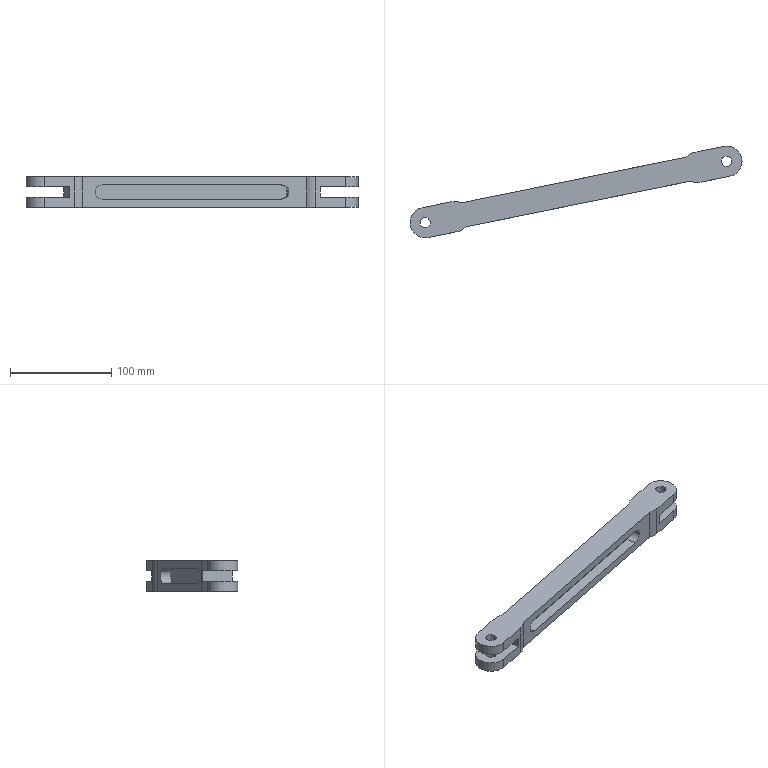Part | SolidWorks | features ICE 2, Extrusion 1, MirrorPattern 1 | 1 solid | 44 faces | box 327.343 x 90.496 x 30 mm | volume 173247 mm3 | cylinder 24 | plane 20 | commonest cylinder face diameters 30 x10 10 x8 14 x6
STEP:
#1=CARTESIAN_POINT('',(680.932,276.249,2993.336));
#2=VERTEX_POINT('',#1);
#3=CARTESIAN_POINT('',(674.073,274.853,2986.336));
#4=VERTEX_POINT('',#3);
#5=CARTESIAN_POINT('',(680.932,276.249,2986.336));
#6=DIRECTION('',(0.1994,-0.9799,0.));
#7=DIRECTION('',(0.9799,0.1994,0.));
#8=AXIS2_PLACEMENT_3D('',#5,#6,#7);
#9=CIRCLE('',#8,7.);
#10=EDGE_CURVE('',#2,#4,#9,.T.);
#11=ORIENTED_EDGE('',*,*,#10,.T.);
#12=CARTESIAN_POINT('',(672.079,284.652,2986.336));
#13=VERTEX_POINT('',#12);
#14=CARTESIAN_POINT('',(674.073,274.853,2986.336));
#15=DIRECTION('',(-0.1994,0.9799,0.));
#16=VECTOR('',#15,1000.);
#17=LINE('',#14,#16);
#18=EDGE_CURVE('',#4,#13,#17,.T.);
#19=ORIENTED_EDGE('',*,*,#18,.T.);
#20=CARTESIAN_POINT('',(678.939,286.048,2993.336));
#21=VERTEX_POINT('',#20);
#22=CARTESIAN_POINT('',(678.939,286.048,2986.336));
#23=DIRECTION('',(0.1994,-0.9799,0.));
#24=DIRECTION('',(0.9799,0.1994,0.));
#25=AXIS2_PLACEMENT_3D('',#22,#23,#24);
#26=CIRCLE('',#25,7.);
#27=EDGE_CURVE('',#21,#13,#26,.T.);
#28=ORIENTED_EDGE('',*,*,#27,.F.);
#29=CARTESIAN_POINT('',(680.932,276.249,2993.336));
#30=DIRECTION('',(-0.1994,0.9799,0.));
#31=VECTOR('',#30,1000.);
#32=LINE('',#29,#31);
#33=EDGE_CURVE('',#2,#21,#32,.T.);
#34=ORIENTED_EDGE('',*,*,#33,.F.);
#35=EDGE_LOOP('',(#11,#19,#28,#34));
#36=FACE_OUTER_BOUND('',#35,.T.);
#37=CARTESIAN_POINT('',(680.932,276.249,2986.336));
#38=DIRECTION('',(-0.1994,0.9799,0.));
#39=DIRECTION('',(-0.9799,-0.1994,0.));
#40=AXIS2_PLACEMENT_3D('',#37,#38,#39);
#41=CYLINDRICAL_SURFACE('',#40,7.);
#42=ADVANCED_FACE('',(#36),#41,.F.);
#43=CARTESIAN_POINT('',(865.742,309.767,2986.336));
#44=VERTEX_POINT('',#43);
#45=CARTESIAN_POINT('',(858.883,308.372,2993.336));
#46=VERTEX_POINT('',#45);
#47=CARTESIAN_POINT('',(858.883,308.372,2986.336));
#48=DIRECTION('',(0.1994,-0.9799,0.));
#49=DIRECTION('',(0.9799,0.1994,0.));
#50=AXIS2_PLACEMENT_3D('',#47,#48,#49);
#51=CIRCLE('',#50,7.);
#52=EDGE_CURVE('',#44,#46,#51,.T.);
#53=ORIENTED_EDGE('',*,*,#52,.F.);
#54=CARTESIAN_POINT('',(867.736,299.968,2986.336));
#55=VERTEX_POINT('',#54);
#56=CARTESIAN_POINT('',(865.742,309.767,2986.336));
#57=DIRECTION('',(0.1994,-0.9799,0.));
#58=VECTOR('',#57,1000.);
#59=LINE('',#56,#58);
#60=EDGE_CURVE('',#44,#55,#59,.T.);
#61=ORIENTED_EDGE('',*,*,#60,.T.);
#62=CARTESIAN_POINT('',(860.876,298.572,2993.336));
#63=VERTEX_POINT('',#62);
#64=CARTESIAN_POINT('',(860.876,298.572,2986.336));
#65=DIRECTION('',(0.1994,-0.9799,0.));
#66=DIRECTION('',(0.9799,0.1994,0.));
#67=AXIS2_PLACEMENT_3D('',#64,#65,#66);
#68=CIRCLE('',#67,7.);
#69=EDGE_CURVE('',#55,#63,#68,.T.);
#70=ORIENTED_EDGE('',*,*,#69,.T.);
#71=CARTESIAN_POINT('',(858.883,308.372,2993.336));
#72=DIRECTION('',(0.1994,-0.9799,0.));
#73=VECTOR('',#72,1000.);
#74=LINE('',#71,#73);
#75=EDGE_CURVE('',#46,#63,#74,.T.);
#76=ORIENTED_EDGE('',*,*,#75,.F.);
#77=EDGE_LOOP('',(#53,#61,#70,#76));
#78=FACE_OUTER_BOUND('',#77,.T.);
#79=CARTESIAN_POINT('',(858.883,308.372,2986.336));
#80=DIRECTION('',(0.1994,-0.9799,0.));
#81=DIRECTION('',(0.9799,0.1994,0.));
#82=AXIS2_PLACEMENT_3D('',#79,#80,#81);
#83=CYLINDRICAL_SURFACE('',#82,7.);
#84=ADVANCED_FACE('',(#78),#83,.F.);
#85=CARTESIAN_POINT('',(925.925,323.036,2991.336));
#86=VERTEX_POINT('',#85);
#87=CARTESIAN_POINT('',(915.925,323.036,2991.336));
#88=VERTEX_POINT('',#87);
#89=CARTESIAN_POINT('',(920.925,323.036,2991.336));
#90=DIRECTION('',(0.,0.,-1.));
#91=DIRECTION('',(1.,0.,0.));
#92=AXIS2_PLACEMENT_3D('',#89,#90,#91);
#93=CIRCLE('',#92,5.);
#94=EDGE_CURVE('',#86,#88,#93,.T.);
#95=ORIENTED_EDGE('',*,*,#94,.T.);
#96=CARTESIAN_POINT('',(915.925,323.036,3001.336));
#97=VERTEX_POINT('',#96);
#98=CARTESIAN_POINT('',(915.925,323.036,2631.714));
#99=DIRECTION('',(0.,0.,1.));
#100=VECTOR('',#99,1000.);
#101=LINE('',#98,#100);
#102=EDGE_CURVE('',#88,#97,#101,.T.);
#103=ORIENTED_EDGE('',*,*,#102,.T.);
#104=CARTESIAN_POINT('',(925.925,323.036,3001.336));
#105=VERTEX_POINT('',#104);
#106=CARTESIAN_POINT('',(920.925,323.036,3001.336));
#107=DIRECTION('',(0.,0.,1.));
#108=DIRECTION('',(1.,0.,0.));
#109=AXIS2_PLACEMENT_3D('',#106,#107,#108);
#110=CIRCLE('',#109,5.);
#111=EDGE_CURVE('',#97,#105,#110,.T.);
#112=ORIENTED_EDGE('',*,*,#111,.T.);
#113=CARTESIAN_POINT('',(925.925,323.036,2631.714));
#114=DIRECTION('',(0.,0.,1.));
#115=VECTOR('',#114,1000.);
#116=LINE('',#113,#115);
#117=EDGE_CURVE('',#86,#105,#116,.T.);
#118=ORIENTED_EDGE('',*,*,#117,.F.);
#119=EDGE_LOOP('',(#95,#103,#112,#118));
#120=FACE_OUTER_BOUND('',#119,.T.);
#121=CARTESIAN_POINT('',(920.925,323.036,2631.714));
#122=DIRECTION('',(0.,0.,1.));
#123=DIRECTION('',(1.,0.,0.));
#124=AXIS2_PLACEMENT_3D('',#121,#122,#123);
#125=CYLINDRICAL_SURFACE('',#124,5.);
#126=ADVANCED_FACE('',(#120),#125,.F.);
#127=CARTESIAN_POINT('',(628.582,262.54,2991.336));
#128=VERTEX_POINT('',#127);
#129=CARTESIAN_POINT('',(618.582,262.54,2991.336));
#130=VERTEX_POINT('',#129);
#131=CARTESIAN_POINT('',(623.582,262.54,2991.336));
#132=DIRECTION('',(0.,0.,-1.));
#133=DIRECTION('',(1.,0.,0.));
#134=AXIS2_PLACEMENT_3D('',#131,#132,#133);
#135=CIRCLE('',#134,5.);
#136=EDGE_CURVE('',#128,#130,#135,.T.);
#137=ORIENTED_EDGE('',*,*,#136,.T.);
#138=CARTESIAN_POINT('',(618.582,262.54,3001.336));
#139=VERTEX_POINT('',#138);
#140=CARTESIAN_POINT('',(618.582,262.54,2631.714));
#141=DIRECTION('',(0.,0.,1.));
#142=VECTOR('',#141,1000.);
#143=LINE('',#140,#142);
#144=EDGE_CURVE('',#130,#139,#143,.T.);
#145=ORIENTED_EDGE('',*,*,#144,.T.);
#146=CARTESIAN_POINT('',(628.582,262.54,3001.336));
#147=VERTEX_POINT('',#146);
#148=CARTESIAN_POINT('',(623.582,262.54,3001.336));
#149=DIRECTION('',(0.,0.,1.));
#150=DIRECTION('',(1.,0.,0.));
#151=AXIS2_PLACEMENT_3D('',#148,#149,#150);
#152=CIRCLE('',#151,5.);
#153=EDGE_CURVE('',#139,#147,#152,.T.);
#154=ORIENTED_EDGE('',*,*,#153,.T.);
#155=CARTESIAN_POINT('',(628.582,262.54,2631.714));
#156=DIRECTION('',(0.,0.,1.));
#157=VECTOR('',#156,1000.);
#158=LINE('',#155,#157);
#159=EDGE_CURVE('',#128,#147,#158,.T.);
#160=ORIENTED_EDGE('',*,*,#159,.F.);
#161=EDGE_LOOP('',(#137,#145,#154,#160));
#162=FACE_OUTER_BOUND('',#161,.T.);
#163=CARTESIAN_POINT('',(623.582,262.54,2631.714));
#164=DIRECTION('',(0.,0.,1.));
#165=DIRECTION('',(1.,0.,0.));
#166=AXIS2_PLACEMENT_3D('',#163,#164,#165);
#167=CYLINDRICAL_SURFACE('',#166,5.);
#168=ADVANCED_FACE('',(#162),#167,.F.);
#169=CARTESIAN_POINT('',(935.925,323.036,2991.336));
#170=VERTEX_POINT('',#169);
#171=CARTESIAN_POINT('',(923.916,308.337,2991.336));
#172=VERTEX_POINT('',#171);
#173=CARTESIAN_POINT('',(920.925,323.036,2991.336));
#174=DIRECTION('',(0.,0.,-1.));
#175=DIRECTION('',(1.,0.,0.));
#176=AXIS2_PLACEMENT_3D('',#173,#174,#175);
#177=CIRCLE('',#176,15.);
#178=EDGE_CURVE('',#170,#172,#177,.T.);
#179=ORIENTED_EDGE('',*,*,#178,.F.);
#180=CARTESIAN_POINT('',(935.925,323.036,3001.336));
#181=VERTEX_POINT('',#180);
#182=CARTESIAN_POINT('',(935.925,323.036,2631.714));
#183=DIRECTION('',(0.,0.,1.));
#184=VECTOR('',#183,1000.);
#185=LINE('',#182,#184);
#186=EDGE_CURVE('',#170,#181,#185,.T.);
#187=ORIENTED_EDGE('',*,*,#186,.T.);
#188=CARTESIAN_POINT('',(923.916,308.337,3001.336));
#189=VERTEX_POINT('',#188);
#190=CARTESIAN_POINT('',(920.925,323.036,3001.336));
#191=DIRECTION('',(0.,0.,1.));
#192=DIRECTION('',(1.,0.,0.));
#193=AXIS2_PLACEMENT_3D('',#190,#191,#192);
#194=CIRCLE('',#193,15.);
#195=EDGE_CURVE('',#189,#181,#194,.T.);
#196=ORIENTED_EDGE('',*,*,#195,.F.);
#197=CARTESIAN_POINT('',(923.916,308.337,2631.714));
#198=DIRECTION('',(0.,0.,1.));
#199=VECTOR('',#198,1000.);
#200=LINE('',#197,#199);
#201=EDGE_CURVE('',#172,#189,#200,.T.);
#202=ORIENTED_EDGE('',*,*,#201,.F.);
#203=EDGE_LOOP('',(#179,#187,#196,#202));
#204=FACE_OUTER_BOUND('',#203,.T.);
#205=CARTESIAN_POINT('',(920.925,323.036,2631.714));
#206=DIRECTION('',(0.,0.,1.));
#207=DIRECTION('',(1.,0.,0.));
#208=AXIS2_PLACEMENT_3D('',#205,#206,#207);
#209=CYLINDRICAL_SURFACE('',#208,15.);
#210=ADVANCED_FACE('',(#204),#209,.T.);
#211=CARTESIAN_POINT('',(925.925,323.036,2971.336));
#212=VERTEX_POINT('',#211);
#213=CARTESIAN_POINT('',(915.925,323.036,2971.336));
#214=VERTEX_POINT('',#213);
#215=CARTESIAN_POINT('',(920.925,323.036,2971.336));
#216=DIRECTION('',(0.,0.,-1.));
#217=DIRECTION('',(1.,0.,0.));
#218=AXIS2_PLACEMENT_3D('',#215,#216,#217);
#219=CIRCLE('',#218,5.);
#220=EDGE_CURVE('',#212,#214,#219,.T.);
#221=ORIENTED_EDGE('',*,*,#220,.T.);
#222=CARTESIAN_POINT('',(915.925,323.036,2981.336));
#223=VERTEX_POINT('',#222);
#224=CARTESIAN_POINT('',(915.925,323.036,2631.714));
#225=DIRECTION('',(0.,0.,1.));
#226=VECTOR('',#225,1000.);
#227=LINE('',#224,#226);
#228=EDGE_CURVE('',#214,#223,#227,.T.);
#229=ORIENTED_EDGE('',*,*,#228,.T.);
#230=CARTESIAN_POINT('',(925.925,323.036,2981.336));
#231=VERTEX_POINT('',#230);
#232=CARTESIAN_POINT('',(920.925,323.036,2981.336));
#233=DIRECTION('',(0.,0.,1.));
#234=DIRECTION('',(-1.,0.,0.));
#235=AXIS2_PLACEMENT_3D('',#232,#233,#234);
#236=CIRCLE('',#235,5.);
#237=EDGE_CURVE('',#223,#231,#236,.T.);
#238=ORIENTED_EDGE('',*,*,#237,.T.);
#239=CARTESIAN_POINT('',(925.925,323.036,2631.714));
#240=DIRECTION('',(0.,0.,1.));
#241=VECTOR('',#240,1000.);
#242=LINE('',#239,#241);
#243=EDGE_CURVE('',#212,#231,#242,.T.);
#244=ORIENTED_EDGE('',*,*,#243,.F.);
#245=EDGE_LOOP('',(#221,#229,#238,#244));
#246=FACE_OUTER_BOUND('',#245,.T.);
#247=CARTESIAN_POINT('',(920.925,323.036,2631.714));
#248=DIRECTION('',(0.,0.,1.));
#249=DIRECTION('',(1.,0.,0.));
#250=AXIS2_PLACEMENT_3D('',#247,#248,#249);
#251=CYLINDRICAL_SURFACE('',#250,5.);
#252=ADVANCED_FACE('',(#246),#251,.F.);
#253=CARTESIAN_POINT('',(628.582,262.54,2971.336));
#254=VERTEX_POINT('',#253);
#255=CARTESIAN_POINT('',(618.582,262.54,2971.336));
#256=VERTEX_POINT('',#255);
#257=CARTESIAN_POINT('',(623.582,262.54,2971.336));
#258=DIRECTION('',(0.,0.,-1.));
#259=DIRECTION('',(1.,0.,0.));
#260=AXIS2_PLACEMENT_3D('',#257,#258,#259);
#261=CIRCLE('',#260,5.);
#262=EDGE_CURVE('',#254,#256,#261,.T.);
#263=ORIENTED_EDGE('',*,*,#262,.T.);
#264=CARTESIAN_POINT('',(618.582,262.54,2981.336));
#265=VERTEX_POINT('',#264);
#266=CARTESIAN_POINT('',(618.582,262.54,2631.714));
#267=DIRECTION('',(0.,0.,1.));
#268=VECTOR('',#267,1000.);
#269=LINE('',#266,#268);
#270=EDGE_CURVE('',#256,#265,#269,.T.);
#271=ORIENTED_EDGE('',*,*,#270,.T.);
#272=CARTESIAN_POINT('',(628.582,262.54,2981.336));
#273=VERTEX_POINT('',#272);
#274=CARTESIAN_POINT('',(623.582,262.54,2981.336));
#275=DIRECTION('',(0.,0.,1.));
#276=DIRECTION('',(-1.,0.,0.));
#277=AXIS2_PLACEMENT_3D('',#274,#275,#276);
#278=CIRCLE('',#277,5.);
#279=EDGE_CURVE('',#265,#273,#278,.T.);
#280=ORIENTED_EDGE('',*,*,#279,.T.);
#281=CARTESIAN_POINT('',(628.582,262.54,2631.714));
#282=DIRECTION('',(0.,0.,1.));
#283=VECTOR('',#282,1000.);
#284=LINE('',#281,#283);
#285=EDGE_CURVE('',#254,#273,#284,.T.);
#286=ORIENTED_EDGE('',*,*,#285,.F.);
#287=EDGE_LOOP('',(#263,#271,#280,#286));
#288=FACE_OUTER_BOUND('',#287,.T.);
#289=CARTESIAN_POINT('',(623.582,262.54,2631.714));
#290=DIRECTION('',(0.,0.,1.));
#291=DIRECTION('',(1.,0.,0.));
#292=AXIS2_PLACEMENT_3D('',#289,#290,#291);
#293=CYLINDRICAL_SURFACE('',#292,5.);
#294=ADVANCED_FACE('',(#288),#293,.F.);
#295=CARTESIAN_POINT('',(935.925,323.036,2971.336));
#296=VERTEX_POINT('',#295);
#297=CARTESIAN_POINT('',(923.916,308.337,2971.336));
#298=VERTEX_POINT('',#297);
#299=CARTESIAN_POINT('',(920.925,323.036,2971.336));
#300=DIRECTION('',(0.,0.,-1.));
#301=DIRECTION('',(1.,0.,0.));
#302=AXIS2_PLACEMENT_3D('',#299,#300,#301);
#303=CIRCLE('',#302,15.);
#304=EDGE_CURVE('',#296,#298,#303,.T.);
#305=ORIENTED_EDGE('',*,*,#304,.F.);
#306=CARTESIAN_POINT('',(935.925,323.036,2981.336));
#307=VERTEX_POINT('',#306);
#308=CARTESIAN_POINT('',(935.925,323.036,2631.714));
#309=DIRECTION('',(0.,0.,1.));
#310=VECTOR('',#309,1000.);
#311=LINE('',#308,#310);
#312=EDGE_CURVE('',#296,#307,#311,.T.);
#313=ORIENTED_EDGE('',*,*,#312,.T.);
#314=CARTESIAN_POINT('',(923.916,308.337,2981.336));
#315=VERTEX_POINT('',#314);
#316=CARTESIAN_POINT('',(920.925,323.036,2981.336));
#317=DIRECTION('',(0.,0.,1.));
#318=DIRECTION('',(-1.,0.,0.));
#319=AXIS2_PLACEMENT_3D('',#316,#317,#318);
#320=CIRCLE('',#319,15.);
#321=EDGE_CURVE('',#315,#307,#320,.T.);
#322=ORIENTED_EDGE('',*,*,#321,.F.);
#323=CARTESIAN_POINT('',(923.916,308.337,2631.714));
#324=DIRECTION('',(0.,0.,1.));
#325=VECTOR('',#324,1000.);
#326=LINE('',#323,#325);
#327=EDGE_CURVE('',#298,#315,#326,.T.);
#328=ORIENTED_EDGE('',*,*,#327,.F.);
#329=EDGE_LOOP('',(#305,#313,#322,#328));
#330=FACE_OUTER_BOUND('',#329,.T.);
#331=CARTESIAN_POINT('',(920.925,323.036,2631.714));
#332=DIRECTION('',(0.,0.,1.));
#333=DIRECTION('',(1.,0.,0.));
#334=AXIS2_PLACEMENT_3D('',#331,#332,#333);
#335=CYLINDRICAL_SURFACE('',#334,15.);
#336=ADVANCED_FACE('',(#330),#335,.T.);
#337=CARTESIAN_POINT('',(659.407,282.074,2971.336));
#338=VERTEX_POINT('',#337);
#339=CARTESIAN_POINT('',(880.316,327.019,2971.336));
#340=VERTEX_POINT('',#339);
#341=CARTESIAN_POINT('',(880.316,327.019,2971.336));
#342=DIRECTION('',(0.9799,0.1994,0.));
#343=VECTOR('',#342,1000.);
#344=LINE('',#341,#343);
#345=EDGE_CURVE('',#338,#340,#344,.T.);
#346=ORIENTED_EDGE('',*,*,#345,.F.);
#347=CARTESIAN_POINT('',(659.407,282.074,3001.336));
#348=VERTEX_POINT('',#347);
#349=CARTESIAN_POINT('',(659.407,282.074,2631.714));
#350=DIRECTION('',(0.,0.,1.));
#351=VECTOR('',#350,1000.);
#352=LINE('',#349,#351);
#353=EDGE_CURVE('',#338,#348,#352,.T.);
#354=ORIENTED_EDGE('',*,*,#353,.T.);
#355=CARTESIAN_POINT('',(880.316,327.019,3001.336));
#356=VERTEX_POINT('',#355);
#357=CARTESIAN_POINT('',(880.316,327.019,3001.336));
#358=DIRECTION('',(-0.9799,-0.1994,0.));
#359=VECTOR('',#358,1000.);
#360=LINE('',#357,#359);
#361=EDGE_CURVE('',#356,#348,#360,.T.);
#362=ORIENTED_EDGE('',*,*,#361,.F.);
#363=CARTESIAN_POINT('',(880.316,327.019,2631.714));
#364=DIRECTION('',(0.,0.,1.));
#365=VECTOR('',#364,1000.);
#366=LINE('',#363,#365);
#367=EDGE_CURVE('',#340,#356,#366,.T.);
#368=ORIENTED_EDGE('',*,*,#367,.F.);
#369=EDGE_LOOP('',(#346,#354,#362,#368));
#370=FACE_OUTER_BOUND('',#369,.T.);
#371=CARTESIAN_POINT('',(856.091,322.091,2993.336));
#372=VERTEX_POINT('',#371);
#373=CARTESIAN_POINT('',(678.939,286.048,2993.336));
#374=DIRECTION('',(-0.9799,-0.1994,0.));
#375=VECTOR('',#374,1000.);
#376=LINE('',#373,#375);
#377=EDGE_CURVE('',#372,#21,#376,.T.);
#378=ORIENTED_EDGE('',*,*,#377,.T.);
#379=ORIENTED_EDGE('',*,*,#27,.T.);
#380=CARTESIAN_POINT('',(678.939,286.048,2979.336));
#381=VERTEX_POINT('',#380);
#382=CARTESIAN_POINT('',(678.939,286.048,2986.336));
#383=DIRECTION('',(0.1994,-0.9799,0.));
#384=DIRECTION('',(0.9799,0.1994,0.));
#385=AXIS2_PLACEMENT_3D('',#382,#383,#384);
#386=CIRCLE('',#385,7.);
#387=EDGE_CURVE('',#13,#381,#386,.T.);
#388=ORIENTED_EDGE('',*,*,#387,.T.);
#389=CARTESIAN_POINT('',(856.091,322.091,2979.336));
#390=VERTEX_POINT('',#389);
#391=CARTESIAN_POINT('',(678.939,286.048,2979.336));
#392=DIRECTION('',(0.9799,0.1994,0.));
#393=VECTOR('',#392,1000.);
#394=LINE('',#391,#393);
#395=EDGE_CURVE('',#381,#390,#394,.T.);
#396=ORIENTED_EDGE('',*,*,#395,.T.);
#397=CARTESIAN_POINT('',(856.091,322.091,2986.336));
#398=DIRECTION('',(0.1994,-0.9799,0.));
#399=DIRECTION('',(0.9799,0.1994,0.));
#400=AXIS2_PLACEMENT_3D('',#397,#398,#399);
#401=CIRCLE('',#400,7.);
#402=EDGE_CURVE('',#390,#372,#401,.T.);
#403=ORIENTED_EDGE('',*,*,#402,.T.);
#404=EDGE_LOOP('',(#378,#379,#388,#396,#403));
#405=FACE_BOUND('',#404,.T.);
#406=CARTESIAN_POINT('',(880.316,327.019,2631.714));
#407=DIRECTION('',(-0.1994,0.9799,0.));
#408=DIRECTION('',(-0.9799,-0.1994,0.));
#409=AXIS2_PLACEMENT_3D('',#406,#407,#408);
#410=PLANE('',#409);
#411=ADVANCED_FACE('',(#370,#405),#410,.T.);
#412=CARTESIAN_POINT('',(620.592,277.238,2981.336));
#413=VERTEX_POINT('',#412);
#414=CARTESIAN_POINT('',(626.573,247.841,2981.336));
#415=VERTEX_POINT('',#414);
#416=CARTESIAN_POINT('',(623.582,262.54,2981.336));
#417=DIRECTION('',(0.,0.,1.));
#418=DIRECTION('',(-1.,0.,0.));
#419=AXIS2_PLACEMENT_3D('',#416,#417,#418);
#420=CIRCLE('',#419,15.);
#421=EDGE_CURVE('',#413,#415,#420,.T.);
#422=ORIENTED_EDGE('',*,*,#421,.F.);
#423=CARTESIAN_POINT('',(620.592,277.238,2971.336));
#424=VERTEX_POINT('',#423);
#425=CARTESIAN_POINT('',(620.592,277.238,2631.714));
#426=DIRECTION('',(0.,0.,1.));
#427=VECTOR('',#426,1000.);
#428=LINE('',#425,#427);
#429=EDGE_CURVE('',#424,#413,#428,.T.);
#430=ORIENTED_EDGE('',*,*,#429,.F.);
#431=CARTESIAN_POINT('',(626.573,247.841,2971.336));
#432=VERTEX_POINT('',#431);
#433=CARTESIAN_POINT('',(623.582,262.54,2971.336));
#434=DIRECTION('',(0.,0.,-1.));
#435=DIRECTION('',(1.,0.,0.));
#436=AXIS2_PLACEMENT_3D('',#433,#434,#435);
#437=CIRCLE('',#436,15.);
#438=EDGE_CURVE('',#432,#424,#437,.T.);
#439=ORIENTED_EDGE('',*,*,#438,.F.);
#440=CARTESIAN_POINT('',(626.573,247.841,2631.714));
#441=DIRECTION('',(0.,0.,1.));
#442=VECTOR('',#441,1000.);
#443=LINE('',#440,#442);
#444=EDGE_CURVE('',#432,#415,#443,.T.);
#445=ORIENTED_EDGE('',*,*,#444,.T.);
#446=EDGE_LOOP('',(#422,#430,#439,#445));
#447=FACE_OUTER_BOUND('',#446,.T.);
#448=CARTESIAN_POINT('',(623.582,262.54,2631.714));
#449=DIRECTION('',(0.,0.,1.));
#450=DIRECTION('',(1.,0.,0.));
#451=AXIS2_PLACEMENT_3D('',#448,#449,#450);
#452=CYLINDRICAL_SURFACE('',#451,15.);
#453=ADVANCED_FACE('',(#447),#452,.T.);
#454=ORIENTED_EDGE('',*,*,#312,.F.);
#455=CARTESIAN_POINT('',(917.935,337.734,2971.336));
#456=VERTEX_POINT('',#455);
#457=CARTESIAN_POINT('',(920.925,323.036,2971.336));
#458=DIRECTION('',(0.,0.,-1.));
#459=DIRECTION('',(1.,0.,0.));
#460=AXIS2_PLACEMENT_3D('',#457,#458,#459);
#461=CIRCLE('',#460,15.);
#462=EDGE_CURVE('',#456,#296,#461,.T.);
#463=ORIENTED_EDGE('',*,*,#462,.F.);
#464=CARTESIAN_POINT('',(917.935,337.734,2981.336));
#465=VERTEX_POINT('',#464);
#466=CARTESIAN_POINT('',(917.935,337.734,2631.714));
#467=DIRECTION('',(0.,0.,1.));
#468=VECTOR('',#467,1000.);
#469=LINE('',#466,#468);
#470=EDGE_CURVE('',#456,#465,#469,.T.);
#471=ORIENTED_EDGE('',*,*,#470,.T.);
#472=CARTESIAN_POINT('',(920.925,323.036,2981.336));
#473=DIRECTION('',(0.,0.,1.));
#474=DIRECTION('',(-1.,0.,0.));
#475=AXIS2_PLACEMENT_3D('',#472,#473,#474);
#476=CIRCLE('',#475,15.);
#477=EDGE_CURVE('',#307,#465,#476,.T.);
#478=ORIENTED_EDGE('',*,*,#477,.F.);
#479=EDGE_LOOP('',(#454,#463,#471,#478));
#480=FACE_OUTER_BOUND('',#479,.T.);
#481=CARTESIAN_POINT('',(920.925,323.036,2631.714));
#482=DIRECTION('',(0.,0.,1.));
#483=DIRECTION('',(1.,0.,0.));
#484=AXIS2_PLACEMENT_3D('',#481,#482,#483);
#485=CYLINDRICAL_SURFACE('',#484,15.);
#486=ADVANCED_FACE('',(#480),#485,.T.);
#487=ORIENTED_EDGE('',*,*,#270,.F.);
#488=CARTESIAN_POINT('',(623.582,262.54,2971.336));
#489=DIRECTION('',(0.,0.,-1.));
#490=DIRECTION('',(1.,0.,0.));
#491=AXIS2_PLACEMENT_3D('',#488,#489,#490);
#492=CIRCLE('',#491,5.);
#493=EDGE_CURVE('',#256,#254,#492,.T.);
#494=ORIENTED_EDGE('',*,*,#493,.T.);
#495=ORIENTED_EDGE('',*,*,#285,.T.);
#496=CARTESIAN_POINT('',(623.582,262.54,2981.336));
#497=DIRECTION('',(0.,0.,1.));
#498=DIRECTION('',(-1.,0.,0.));
#499=AXIS2_PLACEMENT_3D('',#496,#497,#498);
#500=CIRCLE('',#499,5.);
#501=EDGE_CURVE('',#273,#265,#500,.T.);
#502=ORIENTED_EDGE('',*,*,#501,.T.);
#503=EDGE_LOOP('',(#487,#494,#495,#502));
#504=FACE_OUTER_BOUND('',#503,.T.);
#505=CARTESIAN_POINT('',(623.582,262.54,2631.714));
#506=DIRECTION('',(0.,0.,1.));
#507=DIRECTION('',(1.,0.,0.));
#508=AXIS2_PLACEMENT_3D('',#505,#506,#507);
#509=CYLINDRICAL_SURFACE('',#508,5.);
#510=ADVANCED_FACE('',(#504),#509,.F.);
#511=ORIENTED_EDGE('',*,*,#228,.F.);
#512=CARTESIAN_POINT('',(920.925,323.036,2971.336));
#513=DIRECTION('',(0.,0.,-1.));
#514=DIRECTION('',(1.,0.,0.));
#515=AXIS2_PLACEMENT_3D('',#512,#513,#514);
#516=CIRCLE('',#515,5.);
#517=EDGE_CURVE('',#214,#212,#516,.T.);
#518=ORIENTED_EDGE('',*,*,#517,.T.);
#519=ORIENTED_EDGE('',*,*,#243,.T.);
#520=CARTESIAN_POINT('',(920.925,323.036,2981.336));
#521=DIRECTION('',(0.,0.,1.));
#522=DIRECTION('',(-1.,0.,0.));
#523=AXIS2_PLACEMENT_3D('',#520,#521,#522);
#524=CIRCLE('',#523,5.);
#525=EDGE_CURVE('',#231,#223,#524,.T.);
#526=ORIENTED_EDGE('',*,*,#525,.T.);
#527=EDGE_LOOP('',(#511,#518,#519,#526));
#528=FACE_OUTER_BOUND('',#527,.T.);
#529=CARTESIAN_POINT('',(920.925,323.036,2631.714));
#530=DIRECTION('',(0.,0.,1.));
#531=DIRECTION('',(1.,0.,0.));
#532=AXIS2_PLACEMENT_3D('',#529,#530,#531);
#533=CYLINDRICAL_SURFACE('',#532,5.);
#534=ADVANCED_FACE('',(#528),#533,.F.);
#535=CARTESIAN_POINT('',(892.569,332.574,2981.336));
#536=VERTEX_POINT('',#535);
#537=CARTESIAN_POINT('',(917.935,337.734,2981.336));
#538=DIRECTION('',(-0.9799,-0.1994,0.));
#539=VECTOR('',#538,1000.);
#540=LINE('',#537,#539);
#541=EDGE_CURVE('',#465,#536,#540,.T.);
#542=ORIENTED_EDGE('',*,*,#541,.F.);
#543=ORIENTED_EDGE('',*,*,#470,.F.);
#544=CARTESIAN_POINT('',(888.537,331.753,2971.336));
#545=VERTEX_POINT('',#544);
#546=CARTESIAN_POINT('',(917.935,337.734,2971.336));
#547=DIRECTION('',(0.9799,0.1994,0.));
#548=VECTOR('',#547,1000.);
#549=LINE('',#546,#548);
#550=EDGE_CURVE('',#545,#456,#549,.T.);
#551=ORIENTED_EDGE('',*,*,#550,.F.);
#552=CARTESIAN_POINT('',(888.537,331.753,3001.336));
#553=VERTEX_POINT('',#552);
#554=CARTESIAN_POINT('',(888.537,331.753,2631.714));
#555=DIRECTION('',(0.,0.,1.));
#556=VECTOR('',#555,1000.);
#557=LINE('',#554,#556);
#558=EDGE_CURVE('',#545,#553,#557,.T.);
#559=ORIENTED_EDGE('',*,*,#558,.T.);
#560=CARTESIAN_POINT('',(917.935,337.734,3001.336));
#561=VERTEX_POINT('',#560);
#562=CARTESIAN_POINT('',(917.935,337.734,3001.336));
#563=DIRECTION('',(-0.9799,-0.1994,0.));
#564=VECTOR('',#563,1000.);
#565=LINE('',#562,#564);
#566=EDGE_CURVE('',#561,#553,#565,.T.);
#567=ORIENTED_EDGE('',*,*,#566,.F.);
#568=CARTESIAN_POINT('',(917.935,337.734,2991.336));
#569=VERTEX_POINT('',#568);
#570=CARTESIAN_POINT('',(917.935,337.734,2631.714));
#571=DIRECTION('',(0.,0.,1.));
#572=VECTOR('',#571,1000.);
#573=LINE('',#570,#572);
#574=EDGE_CURVE('',#569,#561,#573,.T.);
#575=ORIENTED_EDGE('',*,*,#574,.F.);
#576=CARTESIAN_POINT('',(892.569,332.574,2991.336));
#577=VERTEX_POINT('',#576);
#578=CARTESIAN_POINT('',(917.935,337.734,2991.336));
#579=DIRECTION('',(0.9799,0.1994,0.));
#580=VECTOR('',#579,1000.);
#581=LINE('',#578,#580);
#582=EDGE_CURVE('',#577,#569,#581,.T.);
#583=ORIENTED_EDGE('',*,*,#582,.F.);
#584=CARTESIAN_POINT('',(892.569,332.574,2631.714));
#585=DIRECTION('',(0.,0.,1.));
#586=VECTOR('',#585,1000.);
#587=LINE('',#584,#586);
#588=EDGE_CURVE('',#536,#577,#587,.T.);
#589=ORIENTED_EDGE('',*,*,#588,.F.);
#590=EDGE_LOOP('',(#542,#543,#551,#559,#567,#575,#583,#589));
#591=FACE_OUTER_BOUND('',#590,.T.);
#592=CARTESIAN_POINT('',(917.935,337.734,2631.714));
#593=DIRECTION('',(-0.1994,0.9799,0.));
#594=DIRECTION('',(-0.9799,-0.1994,0.));
#595=AXIS2_PLACEMENT_3D('',#592,#593,#594);
#596=PLANE('',#595);
#597=ADVANCED_FACE('',(#591),#596,.T.);
#598=CARTESIAN_POINT('',(891.528,317.054,2971.336));
#599=DIRECTION('',(0.,0.,-1.));
#600=DIRECTION('',(1.,0.,0.));
#601=AXIS2_PLACEMENT_3D('',#598,#599,#600);
#602=CIRCLE('',#601,15.);
#603=EDGE_CURVE('',#340,#545,#602,.T.);
#604=ORIENTED_EDGE('',*,*,#603,.F.);
#605=ORIENTED_EDGE('',*,*,#367,.T.);
#606=CARTESIAN_POINT('',(891.528,317.054,3001.336));
#607=DIRECTION('',(0.,0.,1.));
#608=DIRECTION('',(1.,0.,0.));
#609=AXIS2_PLACEMENT_3D('',#606,#607,#608);
#610=CIRCLE('',#609,15.);
#611=EDGE_CURVE('',#553,#356,#610,.T.);
#612=ORIENTED_EDGE('',*,*,#611,.F.);
#613=ORIENTED_EDGE('',*,*,#558,.F.);
#614=EDGE_LOOP('',(#604,#605,#612,#613));
#615=FACE_OUTER_BOUND('',#614,.T.);
#616=CARTESIAN_POINT('',(891.528,317.054,2631.714));
#617=DIRECTION('',(0.,0.,1.));
#618=DIRECTION('',(1.,0.,0.));
#619=AXIS2_PLACEMENT_3D('',#616,#617,#618);
#620=CYLINDRICAL_SURFACE('',#619,15.);
#621=ADVANCED_FACE('',(#615),#620,.T.);
#622=CARTESIAN_POINT('',(649.989,283.22,2971.336));
#623=VERTEX_POINT('',#622);
#624=CARTESIAN_POINT('',(652.98,268.521,2971.336));
#625=DIRECTION('',(0.,0.,-1.));
#626=DIRECTION('',(1.,0.,0.));
#627=AXIS2_PLACEMENT_3D('',#624,#625,#626);
#628=CIRCLE('',#627,15.);
#629=EDGE_CURVE('',#623,#338,#628,.T.);
#630=ORIENTED_EDGE('',*,*,#629,.F.);
#631=CARTESIAN_POINT('',(649.989,283.22,3001.336));
#632=VERTEX_POINT('',#631);
#633=CARTESIAN_POINT('',(649.989,283.22,2631.714));
#634=DIRECTION('',(0.,0.,1.));
#635=VECTOR('',#634,1000.);
#636=LINE('',#633,#635);
#637=EDGE_CURVE('',#623,#632,#636,.T.);
#638=ORIENTED_EDGE('',*,*,#637,.T.);
#639=CARTESIAN_POINT('',(652.98,268.521,3001.336));
#640=DIRECTION('',(0.,0.,1.));
#641=DIRECTION('',(1.,0.,0.));
#642=AXIS2_PLACEMENT_3D('',#639,#640,#641);
#643=CIRCLE('',#642,15.);
#644=EDGE_CURVE('',#348,#632,#643,.T.);
#645=ORIENTED_EDGE('',*,*,#644,.F.);
#646=ORIENTED_EDGE('',*,*,#353,.F.);
#647=EDGE_LOOP('',(#630,#638,#645,#646));
#648=FACE_OUTER_BOUND('',#647,.T.);
#649=CARTESIAN_POINT('',(652.98,268.521,2631.714));
#650=DIRECTION('',(0.,0.,1.));
#651=DIRECTION('',(1.,0.,0.));
#652=AXIS2_PLACEMENT_3D('',#649,#650,#651);
#653=CYLINDRICAL_SURFACE('',#652,15.);
#654=ADVANCED_FACE('',(#648),#653,.T.);
#655=CARTESIAN_POINT('',(645.957,282.399,2981.336));
#656=VERTEX_POINT('',#655);
#657=CARTESIAN_POINT('',(649.989,283.22,2981.336));
#658=DIRECTION('',(-0.9799,-0.1994,0.));
#659=VECTOR('',#658,1000.);
#660=LINE('',#657,#659);
#661=EDGE_CURVE('',#656,#413,#660,.T.);
#662=ORIENTED_EDGE('',*,*,#661,.F.);
#663=CARTESIAN_POINT('',(645.957,282.399,2991.336));
#664=VERTEX_POINT('',#663);
#665=CARTESIAN_POINT('',(645.957,282.399,2631.714));
#666=DIRECTION('',(0.,0.,-1.));
#667=VECTOR('',#666,1000.);
#668=LINE('',#665,#667);
#669=EDGE_CURVE('',#664,#656,#668,.T.);
#670=ORIENTED_EDGE('',*,*,#669,.F.);
#671=CARTESIAN_POINT('',(620.592,277.238,2991.336));
#672=VERTEX_POINT('',#671);
#673=CARTESIAN_POINT('',(649.989,283.22,2991.336));
#674=DIRECTION('',(0.9799,0.1994,0.));
#675=VECTOR('',#674,1000.);
#676=LINE('',#673,#675);
#677=EDGE_CURVE('',#672,#664,#676,.T.);
#678=ORIENTED_EDGE('',*,*,#677,.F.);
#679=CARTESIAN_POINT('',(620.592,277.238,3001.336));
#680=VERTEX_POINT('',#679);
#681=CARTESIAN_POINT('',(620.592,277.238,2631.714));
#682=DIRECTION('',(0.,0.,1.));
#683=VECTOR('',#682,1000.);
#684=LINE('',#681,#683);
#685=EDGE_CURVE('',#672,#680,#684,.T.);
#686=ORIENTED_EDGE('',*,*,#685,.T.);
#687=CARTESIAN_POINT('',(649.989,283.22,3001.336));
#688=DIRECTION('',(-0.9799,-0.1994,0.));
#689=VECTOR('',#688,1000.);
#690=LINE('',#687,#689);
#691=EDGE_CURVE('',#632,#680,#690,.T.);
#692=ORIENTED_EDGE('',*,*,#691,.F.);
#693=ORIENTED_EDGE('',*,*,#637,.F.);
#694=CARTESIAN_POINT('',(649.989,283.22,2971.336));
#695=DIRECTION('',(0.9799,0.1994,0.));
#696=VECTOR('',#695,1000.);
#697=LINE('',#694,#696);
#698=EDGE_CURVE('',#424,#623,#697,.T.);
#699=ORIENTED_EDGE('',*,*,#698,.F.);
#700=ORIENTED_EDGE('',*,*,#429,.T.);
#701=EDGE_LOOP('',(#662,#670,#678,#686,#692,#693,#699,#700));
#702=FACE_OUTER_BOUND('',#701,.T.);
#703=CARTESIAN_POINT('',(649.989,283.22,2631.714));
#704=DIRECTION('',(-0.1994,0.9799,0.));
#705=DIRECTION('',(-0.9799,-0.1994,0.));
#706=AXIS2_PLACEMENT_3D('',#703,#704,#705);
#707=PLANE('',#706);
#708=ADVANCED_FACE('',(#702),#707,.T.);
#709=CARTESIAN_POINT('',(626.573,247.841,2991.336));
#710=VERTEX_POINT('',#709);
#711=CARTESIAN_POINT('',(623.582,262.54,2991.336));
#712=DIRECTION('',(0.,0.,-1.));
#713=DIRECTION('',(1.,0.,0.));
#714=AXIS2_PLACEMENT_3D('',#711,#712,#713);
#715=CIRCLE('',#714,15.);
#716=EDGE_CURVE('',#710,#672,#715,.T.);
#717=ORIENTED_EDGE('',*,*,#716,.F.);
#718=CARTESIAN_POINT('',(626.573,247.841,3001.336));
#719=VERTEX_POINT('',#718);
#720=CARTESIAN_POINT('',(626.573,247.841,2631.714));
#721=DIRECTION('',(0.,0.,1.));
#722=VECTOR('',#721,1000.);
#723=LINE('',#720,#722);
#724=EDGE_CURVE('',#710,#719,#723,.T.);
#725=ORIENTED_EDGE('',*,*,#724,.T.);
#726=CARTESIAN_POINT('',(623.582,262.54,3001.336));
#727=DIRECTION('',(0.,0.,1.));
#728=DIRECTION('',(1.,0.,0.));
#729=AXIS2_PLACEMENT_3D('',#726,#727,#728);
#730=CIRCLE('',#729,15.);
#731=EDGE_CURVE('',#680,#719,#730,.T.);
#732=ORIENTED_EDGE('',*,*,#731,.F.);
#733=ORIENTED_EDGE('',*,*,#685,.F.);
#734=EDGE_LOOP('',(#717,#725,#732,#733));
#735=FACE_OUTER_BOUND('',#734,.T.);
#736=CARTESIAN_POINT('',(623.582,262.54,2631.714));
#737=DIRECTION('',(0.,0.,1.));
#738=DIRECTION('',(1.,0.,0.));
#739=AXIS2_PLACEMENT_3D('',#736,#737,#738);
#740=CYLINDRICAL_SURFACE('',#739,15.);
#741=ADVANCED_FACE('',(#735),#740,.T.);
#742=CARTESIAN_POINT('',(651.938,253.001,2981.336));
#743=VERTEX_POINT('',#742);
#744=CARTESIAN_POINT('',(651.938,253.001,2981.336));
#745=DIRECTION('',(0.9799,0.1994,0.));
#746=VECTOR('',#745,1000.);
#747=LINE('',#744,#746);
#748=EDGE_CURVE('',#415,#743,#747,.T.);
#749=ORIENTED_EDGE('',*,*,#748,.F.);
#750=ORIENTED_EDGE('',*,*,#444,.F.);
#751=CARTESIAN_POINT('',(655.97,253.822,2971.336));
#752=VERTEX_POINT('',#751);
#753=CARTESIAN_POINT('',(626.573,247.841,2971.336));
#754=DIRECTION('',(-0.9799,-0.1994,0.));
#755=VECTOR('',#754,1000.);
#756=LINE('',#753,#755);
#757=EDGE_CURVE('',#752,#432,#756,.T.);
#758=ORIENTED_EDGE('',*,*,#757,.F.);
#759=CARTESIAN_POINT('',(655.97,253.822,3001.336));
#760=VERTEX_POINT('',#759);
#761=CARTESIAN_POINT('',(655.97,253.822,2631.714));
#762=DIRECTION('',(0.,0.,1.));
#763=VECTOR('',#762,1000.);
#764=LINE('',#761,#763);
#765=EDGE_CURVE('',#752,#760,#764,.T.);
#766=ORIENTED_EDGE('',*,*,#765,.T.);
#767=CARTESIAN_POINT('',(626.573,247.841,3001.336));
#768=DIRECTION('',(0.9799,0.1994,0.));
#769=VECTOR('',#768,1000.);
#770=LINE('',#767,#769);
#771=EDGE_CURVE('',#719,#760,#770,.T.);
#772=ORIENTED_EDGE('',*,*,#771,.F.);
#773=ORIENTED_EDGE('',*,*,#724,.F.);
#774=CARTESIAN_POINT('',(651.938,253.001,2991.336));
#775=VERTEX_POINT('',#774);
#776=CARTESIAN_POINT('',(651.938,253.001,2991.336));
#777=DIRECTION('',(-0.9799,-0.1994,0.));
#778=VECTOR('',#777,1000.);
#779=LINE('',#776,#778);
#780=EDGE_CURVE('',#775,#710,#779,.T.);
#781=ORIENTED_EDGE('',*,*,#780,.F.);
#782=CARTESIAN_POINT('',(651.938,253.001,2991.336));
#783=DIRECTION('',(0.,0.,1.));
#784=VECTOR('',#783,1000.);
#785=LINE('',#782,#784);
#786=EDGE_CURVE('',#743,#775,#785,.T.);
#787=ORIENTED_EDGE('',*,*,#786,.F.);
#788=EDGE_LOOP('',(#749,#750,#758,#766,#772,#773,#781,#787));
#789=FACE_OUTER_BOUND('',#788,.T.);
#790=CARTESIAN_POINT('',(626.573,247.841,2631.714));
#791=DIRECTION('',(0.1994,-0.9799,0.));
#792=DIRECTION('',(0.9799,0.1994,0.));
#793=AXIS2_PLACEMENT_3D('',#790,#791,#792);
#794=PLANE('',#793);
#795=ADVANCED_FACE('',(#789),#794,.T.);
#796=CARTESIAN_POINT('',(664.192,258.556,2971.336));
#797=VERTEX_POINT('',#796);
#798=CARTESIAN_POINT('',(652.98,268.521,2971.336));
#799=DIRECTION('',(0.,0.,-1.));
#800=DIRECTION('',(1.,0.,0.));
#801=AXIS2_PLACEMENT_3D('',#798,#799,#800);
#802=CIRCLE('',#801,15.);
#803=EDGE_CURVE('',#797,#752,#802,.T.);
#804=ORIENTED_EDGE('',*,*,#803,.F.);
#805=CARTESIAN_POINT('',(664.192,258.556,3001.336));
#806=VERTEX_POINT('',#805);
#807=CARTESIAN_POINT('',(664.192,258.556,2631.714));
#808=DIRECTION('',(0.,0.,1.));
#809=VECTOR('',#808,1000.);
#810=LINE('',#807,#809);
#811=EDGE_CURVE('',#797,#806,#810,.T.);
#812=ORIENTED_EDGE('',*,*,#811,.T.);
#813=CARTESIAN_POINT('',(652.98,268.521,3001.336));
#814=DIRECTION('',(0.,0.,1.));
#815=DIRECTION('',(1.,0.,0.));
#816=AXIS2_PLACEMENT_3D('',#813,#814,#815);
#817=CIRCLE('',#816,15.);
#818=EDGE_CURVE('',#760,#806,#817,.T.);
#819=ORIENTED_EDGE('',*,*,#818,.F.);
#820=ORIENTED_EDGE('',*,*,#765,.F.);
#821=EDGE_LOOP('',(#804,#812,#819,#820));
#822=FACE_OUTER_BOUND('',#821,.T.);
#823=CARTESIAN_POINT('',(652.98,268.521,2631.714));
#824=DIRECTION('',(0.,0.,1.));
#825=DIRECTION('',(1.,0.,0.));
#826=AXIS2_PLACEMENT_3D('',#823,#824,#825);
#827=CYLINDRICAL_SURFACE('',#826,15.);
#828=ADVANCED_FACE('',(#822),#827,.T.);
#829=CARTESIAN_POINT('',(683.724,262.53,2993.336));
#830=VERTEX_POINT('',#829);
#831=CARTESIAN_POINT('',(683.724,262.53,2979.336));
#832=VERTEX_POINT('',#831);
#833=CARTESIAN_POINT('',(683.724,262.53,2986.336));
#834=DIRECTION('',(0.1994,-0.9799,0.));
#835=DIRECTION('',(0.9799,0.1994,0.));
#836=AXIS2_PLACEMENT_3D('',#833,#834,#835);
#837=CIRCLE('',#836,7.);
#838=EDGE_CURVE('',#830,#832,#837,.T.);
#839=ORIENTED_EDGE('',*,*,#838,.F.);
#840=CARTESIAN_POINT('',(683.724,262.53,2993.336));
#841=DIRECTION('',(-0.9799,-0.1994,0.));
#842=VECTOR('',#841,1000.);
#843=LINE('',#840,#842);
#844=EDGE_CURVE('',#63,#830,#843,.T.);
#845=ORIENTED_EDGE('',*,*,#844,.F.);
#846=ORIENTED_EDGE('',*,*,#69,.F.);
#847=CARTESIAN_POINT('',(860.876,298.572,2979.336));
#848=VERTEX_POINT('',#847);
#849=CARTESIAN_POINT('',(860.876,298.572,2986.336));
#850=DIRECTION('',(0.1994,-0.9799,0.));
#851=DIRECTION('',(0.9799,0.1994,0.));
#852=AXIS2_PLACEMENT_3D('',#849,#850,#851);
#853=CIRCLE('',#852,7.);
#854=EDGE_CURVE('',#848,#55,#853,.T.);
#855=ORIENTED_EDGE('',*,*,#854,.F.);
#856=CARTESIAN_POINT('',(683.724,262.53,2979.336));
#857=DIRECTION('',(0.9799,0.1994,0.));
#858=VECTOR('',#857,1000.);
#859=LINE('',#856,#858);
#860=EDGE_CURVE('',#832,#848,#859,.T.);
#861=ORIENTED_EDGE('',*,*,#860,.F.);
#862=EDGE_LOOP('',(#839,#845,#846,#855,#861));
#863=FACE_BOUND('',#862,.T.);
#864=CARTESIAN_POINT('',(885.101,303.501,2971.336));
#865=VERTEX_POINT('',#864);
#866=CARTESIAN_POINT('',(664.192,258.556,2971.336));
#867=DIRECTION('',(-0.9799,-0.1994,0.));
#868=VECTOR('',#867,1000.);
#869=LINE('',#866,#868);
#870=EDGE_CURVE('',#865,#797,#869,.T.);
#871=ORIENTED_EDGE('',*,*,#870,.F.);
#872=CARTESIAN_POINT('',(885.101,303.501,3001.336));
#873=VERTEX_POINT('',#872);
#874=CARTESIAN_POINT('',(885.101,303.501,2631.714));
#875=DIRECTION('',(0.,0.,1.));
#876=VECTOR('',#875,1000.);
#877=LINE('',#874,#876);
#878=EDGE_CURVE('',#865,#873,#877,.T.);
#879=ORIENTED_EDGE('',*,*,#878,.T.);
#880=CARTESIAN_POINT('',(664.192,258.556,3001.336));
#881=DIRECTION('',(0.9799,0.1994,0.));
#882=VECTOR('',#881,1000.);
#883=LINE('',#880,#882);
#884=EDGE_CURVE('',#806,#873,#883,.T.);
#885=ORIENTED_EDGE('',*,*,#884,.F.);
#886=ORIENTED_EDGE('',*,*,#811,.F.);
#887=EDGE_LOOP('',(#871,#879,#885,#886));
#888=FACE_OUTER_BOUND('',#887,.T.);
#889=CARTESIAN_POINT('',(664.192,258.556,2631.714));
#890=DIRECTION('',(0.1994,-0.9799,0.));
#891=DIRECTION('',(0.9799,0.1994,0.));
#892=AXIS2_PLACEMENT_3D('',#889,#890,#891);
#893=PLANE('',#892);
#894=ADVANCED_FACE('',(#863,#888),#893,.T.);
#895=CARTESIAN_POINT('',(894.518,302.356,2971.336));
#896=VERTEX_POINT('',#895);
#897=CARTESIAN_POINT('',(891.528,317.054,2971.336));
#898=DIRECTION('',(0.,0.,-1.));
#899=DIRECTION('',(1.,0.,0.));
#900=AXIS2_PLACEMENT_3D('',#897,#898,#899);
#901=CIRCLE('',#900,15.);
#902=EDGE_CURVE('',#896,#865,#901,.T.);
#903=ORIENTED_EDGE('',*,*,#902,.F.);
#904=CARTESIAN_POINT('',(894.518,302.356,3001.336));
#905=VERTEX_POINT('',#904);
#906=CARTESIAN_POINT('',(894.518,302.356,2631.714));
#907=DIRECTION('',(0.,0.,1.));
#908=VECTOR('',#907,1000.);
#909=LINE('',#906,#908);
#910=EDGE_CURVE('',#896,#905,#909,.T.);
#911=ORIENTED_EDGE('',*,*,#910,.T.);
#912=CARTESIAN_POINT('',(891.528,317.054,3001.336));
#913=DIRECTION('',(0.,0.,1.));
#914=DIRECTION('',(1.,0.,0.));
#915=AXIS2_PLACEMENT_3D('',#912,#913,#914);
#916=CIRCLE('',#915,15.);
#917=EDGE_CURVE('',#873,#905,#916,.T.);
#918=ORIENTED_EDGE('',*,*,#917,.F.);
#919=ORIENTED_EDGE('',*,*,#878,.F.);
#920=EDGE_LOOP('',(#903,#911,#918,#919));
#921=FACE_OUTER_BOUND('',#920,.T.);
#922=CARTESIAN_POINT('',(891.528,317.054,2631.714));
#923=DIRECTION('',(0.,0.,1.));
#924=DIRECTION('',(1.,0.,0.));
#925=AXIS2_PLACEMENT_3D('',#922,#923,#924);
#926=CYLINDRICAL_SURFACE('',#925,15.);
#927=ADVANCED_FACE('',(#921),#926,.T.);
#928=CARTESIAN_POINT('',(898.551,303.176,2981.336));
#929=VERTEX_POINT('',#928);
#930=CARTESIAN_POINT('',(898.551,303.176,2981.336));
#931=DIRECTION('',(0.9799,0.1994,0.));
#932=VECTOR('',#931,1000.);
#933=LINE('',#930,#932);
#934=EDGE_CURVE('',#929,#315,#933,.T.);
#935=ORIENTED_EDGE('',*,*,#934,.F.);
#936=CARTESIAN_POINT('',(898.551,303.176,2991.336));
#937=VERTEX_POINT('',#936);
#938=CARTESIAN_POINT('',(898.551,303.176,2991.336));
#939=DIRECTION('',(0.,0.,-1.));
#940=VECTOR('',#939,1000.);
#941=LINE('',#938,#940);
#942=EDGE_CURVE('',#937,#929,#941,.T.);
#943=ORIENTED_EDGE('',*,*,#942,.F.);
#944=CARTESIAN_POINT('',(898.551,303.176,2991.336));
#945=DIRECTION('',(-0.9799,-0.1994,0.));
#946=VECTOR('',#945,1000.);
#947=LINE('',#944,#946);
#948=EDGE_CURVE('',#172,#937,#947,.T.);
#949=ORIENTED_EDGE('',*,*,#948,.F.);
#950=ORIENTED_EDGE('',*,*,#201,.T.);
#951=CARTESIAN_POINT('',(894.518,302.356,3001.336));
#952=DIRECTION('',(0.9799,0.1994,0.));
#953=VECTOR('',#952,1000.);
#954=LINE('',#951,#953);
#955=EDGE_CURVE('',#905,#189,#954,.T.);
#956=ORIENTED_EDGE('',*,*,#955,.F.);
#957=ORIENTED_EDGE('',*,*,#910,.F.);
#958=CARTESIAN_POINT('',(894.518,302.356,2971.336));
#959=DIRECTION('',(-0.9799,-0.1994,0.));
#960=VECTOR('',#959,1000.);
#961=LINE('',#958,#960);
#962=EDGE_CURVE('',#298,#896,#961,.T.);
#963=ORIENTED_EDGE('',*,*,#962,.F.);
#964=ORIENTED_EDGE('',*,*,#327,.T.);
#965=EDGE_LOOP('',(#935,#943,#949,#950,#956,#957,#963,#964));
#966=FACE_OUTER_BOUND('',#965,.T.);
#967=CARTESIAN_POINT('',(894.518,302.356,2631.714));
#968=DIRECTION('',(0.1994,-0.9799,0.));
#969=DIRECTION('',(0.9799,0.1994,0.));
#970=AXIS2_PLACEMENT_3D('',#967,#968,#969);
#971=PLANE('',#970);
#972=ADVANCED_FACE('',(#966),#971,.T.);
#973=ORIENTED_EDGE('',*,*,#186,.F.);
#974=CARTESIAN_POINT('',(920.925,323.036,2991.336));
#975=DIRECTION('',(0.,0.,-1.));
#976=DIRECTION('',(1.,0.,0.));
#977=AXIS2_PLACEMENT_3D('',#974,#975,#976);
#978=CIRCLE('',#977,15.);
#979=EDGE_CURVE('',#569,#170,#978,.T.);
#980=ORIENTED_EDGE('',*,*,#979,.F.);
#981=ORIENTED_EDGE('',*,*,#574,.T.);
#982=CARTESIAN_POINT('',(920.925,323.036,3001.336));
#983=DIRECTION('',(0.,0.,1.));
#984=DIRECTION('',(1.,0.,0.));
#985=AXIS2_PLACEMENT_3D('',#982,#983,#984);
#986=CIRCLE('',#985,15.);
#987=EDGE_CURVE('',#181,#561,#986,.T.);
#988=ORIENTED_EDGE('',*,*,#987,.F.);
#989=EDGE_LOOP('',(#973,#980,#981,#988));
#990=FACE_OUTER_BOUND('',#989,.T.);
#991=CARTESIAN_POINT('',(920.925,323.036,2631.714));
#992=DIRECTION('',(0.,0.,1.));
#993=DIRECTION('',(1.,0.,0.));
#994=AXIS2_PLACEMENT_3D('',#991,#992,#993);
#995=CYLINDRICAL_SURFACE('',#994,15.);
#996=ADVANCED_FACE('',(#990),#995,.T.);
#997=ORIENTED_EDGE('',*,*,#144,.F.);
#998=CARTESIAN_POINT('',(623.582,262.54,2991.336));
#999=DIRECTION('',(0.,0.,-1.));
#1000=DIRECTION('',(1.,0.,0.));
#1001=AXIS2_PLACEMENT_3D('',#998,#999,#1000);
#1002=CIRCLE('',#1001,5.);
#1003=EDGE_CURVE('',#130,#128,#1002,.T.);
#1004=ORIENTED_EDGE('',*,*,#1003,.T.);
#1005=ORIENTED_EDGE('',*,*,#159,.T.);
#1006=CARTESIAN_POINT('',(623.582,262.54,3001.336));
#1007=DIRECTION('',(0.,0.,1.));
#1008=DIRECTION('',(1.,0.,0.));
#1009=AXIS2_PLACEMENT_3D('',#1006,#1007,#1008);
#1010=CIRCLE('',#1009,5.);
#1011=EDGE_CURVE('',#147,#139,#1010,.T.);
#1012=ORIENTED_EDGE('',*,*,#1011,.T.);
#1013=EDGE_LOOP('',(#997,#1004,#1005,#1012));
#1014=FACE_OUTER_BOUND('',#1013,.T.);
#1015=CARTESIAN_POINT('',(623.582,262.54,2631.714));
#1016=DIRECTION('',(0.,0.,1.));
#1017=DIRECTION('',(1.,0.,0.));
#1018=AXIS2_PLACEMENT_3D('',#1015,#1016,#1017);
#1019=CYLINDRICAL_SURFACE('',#1018,5.);
#1020=ADVANCED_FACE('',(#1014),#1019,.F.);
#1021=CARTESIAN_POINT('',(920.925,323.036,3001.336));
#1022=DIRECTION('',(0.,0.,1.));
#1023=DIRECTION('',(1.,0.,0.));
#1024=AXIS2_PLACEMENT_3D('',#1021,#1022,#1023);
#1025=CIRCLE('',#1024,5.);
#1026=EDGE_CURVE('',#105,#97,#1025,.T.);
#1027=ORIENTED_EDGE('',*,*,#1026,.F.);
#1028=ORIENTED_EDGE('',*,*,#111,.F.);
#1029=EDGE_LOOP('',(#1027,#1028));
#1030=FACE_BOUND('',#1029,.T.);
#1031=ORIENTED_EDGE('',*,*,#1011,.F.);
#1032=ORIENTED_EDGE('',*,*,#153,.F.);
#1033=EDGE_LOOP('',(#1031,#1032));
#1034=FACE_BOUND('',#1033,.T.);
#1035=ORIENTED_EDGE('',*,*,#195,.T.);
#1036=ORIENTED_EDGE('',*,*,#987,.T.);
#1037=ORIENTED_EDGE('',*,*,#566,.T.);
#1038=ORIENTED_EDGE('',*,*,#611,.T.);
#1039=ORIENTED_EDGE('',*,*,#361,.T.);
#1040=ORIENTED_EDGE('',*,*,#644,.T.);
#1041=ORIENTED_EDGE('',*,*,#691,.T.);
#1042=ORIENTED_EDGE('',*,*,#731,.T.);
#1043=ORIENTED_EDGE('',*,*,#771,.T.);
#1044=ORIENTED_EDGE('',*,*,#818,.T.);
#1045=ORIENTED_EDGE('',*,*,#884,.T.);
#1046=ORIENTED_EDGE('',*,*,#917,.T.);
#1047=ORIENTED_EDGE('',*,*,#955,.T.);
#1048=EDGE_LOOP('',(#1035,#1036,#1037,#1038,#1039,#1040,#1041,#1042,#1043,#1044,#1045,#1046,#1047));
#1049=FACE_OUTER_BOUND('',#1048,.T.);
#1050=CARTESIAN_POINT('',(920.925,323.036,3001.336));
#1051=DIRECTION('',(0.,0.,1.));
#1052=DIRECTION('',(1.,0.,0.));
#1053=AXIS2_PLACEMENT_3D('',#1050,#1051,#1052);
#1054=PLANE('',#1053);
#1055=ADVANCED_FACE('',(#1030,#1034,#1049),#1054,.T.);
#1056=ORIENTED_EDGE('',*,*,#102,.F.);
#1057=CARTESIAN_POINT('',(920.925,323.036,2991.336));
#1058=DIRECTION('',(0.,0.,-1.));
#1059=DIRECTION('',(1.,0.,0.));
#1060=AXIS2_PLACEMENT_3D('',#1057,#1058,#1059);
#1061=CIRCLE('',#1060,5.);
#1062=EDGE_CURVE('',#88,#86,#1061,.T.);
#1063=ORIENTED_EDGE('',*,*,#1062,.T.);
#1064=ORIENTED_EDGE('',*,*,#117,.T.);
#1065=ORIENTED_EDGE('',*,*,#1026,.T.);
#1066=EDGE_LOOP('',(#1056,#1063,#1064,#1065));
#1067=FACE_OUTER_BOUND('',#1066,.T.);
#1068=CARTESIAN_POINT('',(920.925,323.036,2631.714));
#1069=DIRECTION('',(0.,0.,1.));
#1070=DIRECTION('',(1.,0.,0.));
#1071=AXIS2_PLACEMENT_3D('',#1068,#1069,#1070);
#1072=CYLINDRICAL_SURFACE('',#1071,5.);
#1073=ADVANCED_FACE('',(#1067),#1072,.F.);
#1074=ORIENTED_EDGE('',*,*,#462,.T.);
#1075=ORIENTED_EDGE('',*,*,#304,.T.);
#1076=ORIENTED_EDGE('',*,*,#962,.T.);
#1077=ORIENTED_EDGE('',*,*,#902,.T.);
#1078=ORIENTED_EDGE('',*,*,#870,.T.);
#1079=ORIENTED_EDGE('',*,*,#803,.T.);
#1080=ORIENTED_EDGE('',*,*,#757,.T.);
#1081=ORIENTED_EDGE('',*,*,#438,.T.);
#1082=ORIENTED_EDGE('',*,*,#698,.T.);
#1083=ORIENTED_EDGE('',*,*,#629,.T.);
#1084=ORIENTED_EDGE('',*,*,#345,.T.);
#1085=ORIENTED_EDGE('',*,*,#603,.T.);
#1086=ORIENTED_EDGE('',*,*,#550,.T.);
#1087=EDGE_LOOP('',(#1074,#1075,#1076,#1077,#1078,#1079,#1080,#1081,#1082,#1083,#1084,#1085,#1086));
#1088=FACE_OUTER_BOUND('',#1087,.T.);
#1089=ORIENTED_EDGE('',*,*,#220,.F.);
#1090=ORIENTED_EDGE('',*,*,#517,.F.);
#1091=EDGE_LOOP('',(#1089,#1090));
#1092=FACE_BOUND('',#1091,.T.);
#1093=ORIENTED_EDGE('',*,*,#262,.F.);
#1094=ORIENTED_EDGE('',*,*,#493,.F.);
#1095=EDGE_LOOP('',(#1093,#1094));
#1096=FACE_BOUND('',#1095,.T.);
#1097=CARTESIAN_POINT('',(623.582,262.54,2971.336));
#1098=DIRECTION('',(0.,0.,1.));
#1099=DIRECTION('',(0.9799,0.1994,0.));
#1100=AXIS2_PLACEMENT_3D('',#1097,#1098,#1099);
#1101=PLANE('',#1100);
#1102=ADVANCED_FACE('',(#1088,#1092,#1096),#1101,.F.);
#1103=ORIENTED_EDGE('',*,*,#541,.T.);
#1104=CARTESIAN_POINT('',(882.601,381.57,2981.336));
#1105=DIRECTION('',(0.1994,-0.9799,0.));
#1106=VECTOR('',#1105,1000.);
#1107=LINE('',#1104,#1106);
#1108=EDGE_CURVE('',#536,#929,#1107,.T.);
#1109=ORIENTED_EDGE('',*,*,#1108,.T.);
#1110=ORIENTED_EDGE('',*,*,#934,.T.);
#1111=ORIENTED_EDGE('',*,*,#321,.T.);
#1112=ORIENTED_EDGE('',*,*,#477,.T.);
#1113=EDGE_LOOP('',(#1103,#1109,#1110,#1111,#1112));
#1114=FACE_OUTER_BOUND('',#1113,.T.);
#1115=ORIENTED_EDGE('',*,*,#525,.F.);
#1116=ORIENTED_EDGE('',*,*,#237,.F.);
#1117=EDGE_LOOP('',(#1115,#1116));
#1118=FACE_BOUND('',#1117,.T.);
#1119=CARTESIAN_POINT('',(882.601,381.57,2981.336));
#1120=DIRECTION('',(0.,0.,-1.));
#1121=DIRECTION('',(-1.,0.,0.));
#1122=AXIS2_PLACEMENT_3D('',#1119,#1120,#1121);
#1123=PLANE('',#1122);
#1124=ADVANCED_FACE('',(#1114,#1118),#1123,.F.);
#1125=ORIENTED_EDGE('',*,*,#582,.T.);
#1126=ORIENTED_EDGE('',*,*,#979,.T.);
#1127=ORIENTED_EDGE('',*,*,#178,.T.);
#1128=ORIENTED_EDGE('',*,*,#948,.T.);
#1129=CARTESIAN_POINT('',(882.601,381.57,2991.336));
#1130=DIRECTION('',(0.1994,-0.9799,0.));
#1131=VECTOR('',#1130,1000.);
#1132=LINE('',#1129,#1131);
#1133=EDGE_CURVE('',#577,#937,#1132,.T.);
#1134=ORIENTED_EDGE('',*,*,#1133,.F.);
#1135=EDGE_LOOP('',(#1125,#1126,#1127,#1128,#1134));
#1136=FACE_OUTER_BOUND('',#1135,.T.);
#1137=ORIENTED_EDGE('',*,*,#94,.F.);
#1138=ORIENTED_EDGE('',*,*,#1062,.F.);
#1139=EDGE_LOOP('',(#1137,#1138));
#1140=FACE_BOUND('',#1139,.T.);
#1141=CARTESIAN_POINT('',(882.601,381.57,2991.336));
#1142=DIRECTION('',(0.,0.,1.));
#1143=DIRECTION('',(1.,0.,0.));
#1144=AXIS2_PLACEMENT_3D('',#1141,#1142,#1143);
#1145=PLANE('',#1144);
#1146=ADVANCED_FACE('',(#1136,#1140),#1145,.F.);
#1147=ORIENTED_EDGE('',*,*,#588,.T.);
#1148=ORIENTED_EDGE('',*,*,#1133,.T.);
#1149=ORIENTED_EDGE('',*,*,#942,.T.);
#1150=ORIENTED_EDGE('',*,*,#1108,.F.);
#1151=EDGE_LOOP('',(#1147,#1148,#1149,#1150));
#1152=FACE_OUTER_BOUND('',#1151,.T.);
#1153=CARTESIAN_POINT('',(882.601,381.57,2991.336));
#1154=DIRECTION('',(-0.9799,-0.1994,0.));
#1155=DIRECTION('',(0.1994,-0.9799,0.));
#1156=AXIS2_PLACEMENT_3D('',#1153,#1154,#1155);
#1157=PLANE('',#1156);
#1158=ADVANCED_FACE('',(#1152),#1157,.F.);
#1159=ORIENTED_EDGE('',*,*,#661,.T.);
#1160=ORIENTED_EDGE('',*,*,#421,.T.);
#1161=ORIENTED_EDGE('',*,*,#748,.T.);
#1162=CARTESIAN_POINT('',(635.989,331.395,2981.336));
#1163=DIRECTION('',(0.1994,-0.9799,0.));
#1164=VECTOR('',#1163,1000.);
#1165=LINE('',#1162,#1164);
#1166=EDGE_CURVE('',#656,#743,#1165,.T.);
#1167=ORIENTED_EDGE('',*,*,#1166,.F.);
#1168=EDGE_LOOP('',(#1159,#1160,#1161,#1167));
#1169=FACE_OUTER_BOUND('',#1168,.T.);
#1170=ORIENTED_EDGE('',*,*,#501,.F.);
#1171=ORIENTED_EDGE('',*,*,#279,.F.);
#1172=EDGE_LOOP('',(#1170,#1171));
#1173=FACE_BOUND('',#1172,.T.);
#1174=CARTESIAN_POINT('',(635.989,331.395,2981.336));
#1175=DIRECTION('',(0.,0.,-1.));
#1176=DIRECTION('',(-1.,0.,0.));
#1177=AXIS2_PLACEMENT_3D('',#1174,#1175,#1176);
#1178=PLANE('',#1177);
#1179=ADVANCED_FACE('',(#1169,#1173),#1178,.F.);
#1180=ORIENTED_EDGE('',*,*,#677,.T.);
#1181=CARTESIAN_POINT('',(635.989,331.395,2991.336));
#1182=DIRECTION('',(0.1994,-0.9799,0.));
#1183=VECTOR('',#1182,1000.);
#1184=LINE('',#1181,#1183);
#1185=EDGE_CURVE('',#664,#775,#1184,.T.);
#1186=ORIENTED_EDGE('',*,*,#1185,.T.);
#1187=ORIENTED_EDGE('',*,*,#780,.T.);
#1188=ORIENTED_EDGE('',*,*,#716,.T.);
#1189=EDGE_LOOP('',(#1180,#1186,#1187,#1188));
#1190=FACE_OUTER_BOUND('',#1189,.T.);
#1191=ORIENTED_EDGE('',*,*,#136,.F.);
#1192=ORIENTED_EDGE('',*,*,#1003,.F.);
#1193=EDGE_LOOP('',(#1191,#1192));
#1194=FACE_BOUND('',#1193,.T.);
#1195=CARTESIAN_POINT('',(635.989,331.395,2991.336));
#1196=DIRECTION('',(0.,0.,1.));
#1197=DIRECTION('',(1.,0.,0.));
#1198=AXIS2_PLACEMENT_3D('',#1195,#1196,#1197);
#1199=PLANE('',#1198);
#1200=ADVANCED_FACE('',(#1190,#1194),#1199,.F.);
#1201=ORIENTED_EDGE('',*,*,#669,.T.);
#1202=ORIENTED_EDGE('',*,*,#1166,.T.);
#1203=ORIENTED_EDGE('',*,*,#786,.T.);
#1204=ORIENTED_EDGE('',*,*,#1185,.F.);
#1205=EDGE_LOOP('',(#1201,#1202,#1203,#1204));
#1206=FACE_OUTER_BOUND('',#1205,.T.);
#1207=CARTESIAN_POINT('',(635.989,331.395,2991.336));
#1208=DIRECTION('',(0.9799,0.1994,0.));
#1209=DIRECTION('',(-0.1994,0.9799,0.));
#1210=AXIS2_PLACEMENT_3D('',#1207,#1208,#1209);
#1211=PLANE('',#1210);
#1212=ADVANCED_FACE('',(#1206),#1211,.F.);
#1213=ORIENTED_EDGE('',*,*,#838,.T.);
#1214=CARTESIAN_POINT('',(681.73,272.329,2979.336));
#1215=VERTEX_POINT('',#1214);
#1216=CARTESIAN_POINT('',(681.73,272.329,2979.336));
#1217=DIRECTION('',(0.1994,-0.9799,0.));
#1218=VECTOR('',#1217,1000.);
#1219=LINE('',#1216,#1218);
#1220=EDGE_CURVE('',#1215,#832,#1219,.T.);
#1221=ORIENTED_EDGE('',*,*,#1220,.F.);
#1222=CARTESIAN_POINT('',(681.73,272.329,2993.336));
#1223=VERTEX_POINT('',#1222);
#1224=CARTESIAN_POINT('',(681.73,272.329,2986.336));
#1225=DIRECTION('',(0.1994,-0.9799,0.));
#1226=DIRECTION('',(0.9799,0.1994,0.));
#1227=AXIS2_PLACEMENT_3D('',#1224,#1225,#1226);
#1228=CIRCLE('',#1227,7.);
#1229=EDGE_CURVE('',#1223,#1215,#1228,.T.);
#1230=ORIENTED_EDGE('',*,*,#1229,.F.);
#1231=CARTESIAN_POINT('',(681.73,272.329,2993.336));
#1232=DIRECTION('',(0.1994,-0.9799,0.));
#1233=VECTOR('',#1232,1000.);
#1234=LINE('',#1231,#1233);
#1235=EDGE_CURVE('',#1223,#830,#1234,.T.);
#1236=ORIENTED_EDGE('',*,*,#1235,.T.);
#1237=EDGE_LOOP('',(#1213,#1221,#1230,#1236));
#1238=FACE_OUTER_BOUND('',#1237,.T.);
#1239=CARTESIAN_POINT('',(681.73,272.329,2986.336));
#1240=DIRECTION('',(0.1994,-0.9799,0.));
#1241=DIRECTION('',(0.9799,0.1994,0.));
#1242=AXIS2_PLACEMENT_3D('',#1239,#1240,#1241);
#1243=CYLINDRICAL_SURFACE('',#1242,7.);
#1244=ADVANCED_FACE('',(#1238),#1243,.F.);
#1245=ORIENTED_EDGE('',*,*,#844,.T.);
#1246=ORIENTED_EDGE('',*,*,#1235,.F.);
#1247=CARTESIAN_POINT('',(681.73,272.329,2993.336));
#1248=DIRECTION('',(-0.9799,-0.1994,0.));
#1249=VECTOR('',#1248,1000.);
#1250=LINE('',#1247,#1249);
#1251=EDGE_CURVE('',#46,#1223,#1250,.T.);
#1252=ORIENTED_EDGE('',*,*,#1251,.F.);
#1253=ORIENTED_EDGE('',*,*,#75,.T.);
#1254=EDGE_LOOP('',(#1245,#1246,#1252,#1253));
#1255=FACE_OUTER_BOUND('',#1254,.T.);
#1256=CARTESIAN_POINT('',(681.73,272.329,2993.336));
#1257=DIRECTION('',(0.,0.,1.));
#1258=DIRECTION('',(1.,0.,0.));
#1259=AXIS2_PLACEMENT_3D('',#1256,#1257,#1258);
#1260=PLANE('',#1259);
#1261=ADVANCED_FACE('',(#1255),#1260,.F.);
#1262=ORIENTED_EDGE('',*,*,#60,.F.);
#1263=CARTESIAN_POINT('',(858.883,308.372,2979.336));
#1264=VERTEX_POINT('',#1263);
#1265=CARTESIAN_POINT('',(858.883,308.372,2986.336));
#1266=DIRECTION('',(0.1994,-0.9799,0.));
#1267=DIRECTION('',(0.9799,0.1994,0.));
#1268=AXIS2_PLACEMENT_3D('',#1265,#1266,#1267);
#1269=CIRCLE('',#1268,7.);
#1270=EDGE_CURVE('',#1264,#44,#1269,.T.);
#1271=ORIENTED_EDGE('',*,*,#1270,.F.);
#1272=CARTESIAN_POINT('',(858.883,308.372,2979.336));
#1273=DIRECTION('',(0.1994,-0.9799,0.));
#1274=VECTOR('',#1273,1000.);
#1275=LINE('',#1272,#1274);
#1276=EDGE_CURVE('',#1264,#848,#1275,.T.);
#1277=ORIENTED_EDGE('',*,*,#1276,.T.);
#1278=ORIENTED_EDGE('',*,*,#854,.T.);
#1279=EDGE_LOOP('',(#1262,#1271,#1277,#1278));
#1280=FACE_OUTER_BOUND('',#1279,.T.);
#1281=CARTESIAN_POINT('',(858.883,308.372,2986.336));
#1282=DIRECTION('',(0.1994,-0.9799,0.));
#1283=DIRECTION('',(0.9799,0.1994,0.));
#1284=AXIS2_PLACEMENT_3D('',#1281,#1282,#1283);
#1285=CYLINDRICAL_SURFACE('',#1284,7.);
#1286=ADVANCED_FACE('',(#1280),#1285,.F.);
#1287=ORIENTED_EDGE('',*,*,#860,.T.);
#1288=ORIENTED_EDGE('',*,*,#1276,.F.);
#1289=CARTESIAN_POINT('',(681.73,272.329,2979.336));
#1290=DIRECTION('',(0.9799,0.1994,0.));
#1291=VECTOR('',#1290,1000.);
#1292=LINE('',#1289,#1291);
#1293=EDGE_CURVE('',#1215,#1264,#1292,.T.);
#1294=ORIENTED_EDGE('',*,*,#1293,.F.);
#1295=ORIENTED_EDGE('',*,*,#1220,.T.);
#1296=EDGE_LOOP('',(#1287,#1288,#1294,#1295));
#1297=FACE_OUTER_BOUND('',#1296,.T.);
#1298=CARTESIAN_POINT('',(681.73,272.329,2979.336));
#1299=DIRECTION('',(0.,0.,-1.));
#1300=DIRECTION('',(-1.,0.,0.));
#1301=AXIS2_PLACEMENT_3D('',#1298,#1299,#1300);
#1302=PLANE('',#1301);
#1303=ADVANCED_FACE('',(#1297),#1302,.F.);
#1304=ORIENTED_EDGE('',*,*,#1229,.T.);
#1305=ORIENTED_EDGE('',*,*,#1293,.T.);
#1306=ORIENTED_EDGE('',*,*,#1270,.T.);
#1307=ORIENTED_EDGE('',*,*,#52,.T.);
#1308=ORIENTED_EDGE('',*,*,#1251,.T.);
#1309=EDGE_LOOP('',(#1304,#1305,#1306,#1307,#1308));
#1310=FACE_OUTER_BOUND('',#1309,.T.);
#1311=CARTESIAN_POINT('',(681.73,272.329,2986.336));
#1312=DIRECTION('',(0.1994,-0.9799,0.));
#1313=DIRECTION('',(0.9799,0.1994,0.));
#1314=AXIS2_PLACEMENT_3D('',#1311,#1312,#1313);
#1315=PLANE('',#1314);
#1316=ADVANCED_FACE('',(#1310),#1315,.T.);
#1317=ORIENTED_EDGE('',*,*,#18,.F.);
#1318=CARTESIAN_POINT('',(680.932,276.249,2979.336));
#1319=VERTEX_POINT('',#1318);
#1320=CARTESIAN_POINT('',(680.932,276.249,2986.336));
#1321=DIRECTION('',(0.1994,-0.9799,0.));
#1322=DIRECTION('',(0.9799,0.1994,0.));
#1323=AXIS2_PLACEMENT_3D('',#1320,#1321,#1322);
#1324=CIRCLE('',#1323,7.);
#1325=EDGE_CURVE('',#4,#1319,#1324,.T.);
#1326=ORIENTED_EDGE('',*,*,#1325,.T.);
#1327=CARTESIAN_POINT('',(680.932,276.249,2979.336));
#1328=DIRECTION('',(-0.1994,0.9799,0.));
#1329=VECTOR('',#1328,1000.);
#1330=LINE('',#1327,#1329);
#1331=EDGE_CURVE('',#1319,#381,#1330,.T.);
#1332=ORIENTED_EDGE('',*,*,#1331,.T.);
#1333=ORIENTED_EDGE('',*,*,#387,.F.);
#1334=EDGE_LOOP('',(#1317,#1326,#1332,#1333));
#1335=FACE_OUTER_BOUND('',#1334,.T.);
#1336=CARTESIAN_POINT('',(680.932,276.249,2986.336));
#1337=DIRECTION('',(-0.1994,0.9799,0.));
#1338=DIRECTION('',(-0.9799,-0.1994,0.));
#1339=AXIS2_PLACEMENT_3D('',#1336,#1337,#1338);
#1340=CYLINDRICAL_SURFACE('',#1339,7.);
#1341=ADVANCED_FACE('',(#1335),#1340,.F.);
#1342=ORIENTED_EDGE('',*,*,#395,.F.);
#1343=ORIENTED_EDGE('',*,*,#1331,.F.);
#1344=CARTESIAN_POINT('',(858.085,312.291,2979.336));
#1345=VERTEX_POINT('',#1344);
#1346=CARTESIAN_POINT('',(680.932,276.249,2979.336));
#1347=DIRECTION('',(0.9799,0.1994,0.));
#1348=VECTOR('',#1347,1000.);
#1349=LINE('',#1346,#1348);
#1350=EDGE_CURVE('',#1319,#1345,#1349,.T.);
#1351=ORIENTED_EDGE('',*,*,#1350,.T.);
#1352=CARTESIAN_POINT('',(858.085,312.291,2979.336));
#1353=DIRECTION('',(-0.1994,0.9799,0.));
#1354=VECTOR('',#1353,1000.);
#1355=LINE('',#1352,#1354);
#1356=EDGE_CURVE('',#1345,#390,#1355,.T.);
#1357=ORIENTED_EDGE('',*,*,#1356,.T.);
#1358=EDGE_LOOP('',(#1342,#1343,#1351,#1357));
#1359=FACE_OUTER_BOUND('',#1358,.T.);
#1360=CARTESIAN_POINT('',(680.932,276.249,2979.336));
#1361=DIRECTION('',(0.,0.,1.));
#1362=DIRECTION('',(1.,0.,0.));
#1363=AXIS2_PLACEMENT_3D('',#1360,#1361,#1362);
#1364=PLANE('',#1363);
#1365=ADVANCED_FACE('',(#1359),#1364,.T.);
#1366=ORIENTED_EDGE('',*,*,#402,.F.);
#1367=ORIENTED_EDGE('',*,*,#1356,.F.);
#1368=CARTESIAN_POINT('',(858.085,312.291,2993.336));
#1369=VERTEX_POINT('',#1368);
#1370=CARTESIAN_POINT('',(858.085,312.291,2986.336));
#1371=DIRECTION('',(0.1994,-0.9799,0.));
#1372=DIRECTION('',(0.9799,0.1994,0.));
#1373=AXIS2_PLACEMENT_3D('',#1370,#1371,#1372);
#1374=CIRCLE('',#1373,7.);
#1375=EDGE_CURVE('',#1345,#1369,#1374,.T.);
#1376=ORIENTED_EDGE('',*,*,#1375,.T.);
#1377=CARTESIAN_POINT('',(858.085,312.291,2993.336));
#1378=DIRECTION('',(-0.1994,0.9799,0.));
#1379=VECTOR('',#1378,1000.);
#1380=LINE('',#1377,#1379);
#1381=EDGE_CURVE('',#1369,#372,#1380,.T.);
#1382=ORIENTED_EDGE('',*,*,#1381,.T.);
#1383=EDGE_LOOP('',(#1366,#1367,#1376,#1382));
#1384=FACE_OUTER_BOUND('',#1383,.T.);
#1385=CARTESIAN_POINT('',(858.085,312.291,2986.336));
#1386=DIRECTION('',(-0.1994,0.9799,0.));
#1387=DIRECTION('',(-0.9799,-0.1994,0.));
#1388=AXIS2_PLACEMENT_3D('',#1385,#1386,#1387);
#1389=CYLINDRICAL_SURFACE('',#1388,7.);
#1390=ADVANCED_FACE('',(#1384),#1389,.F.);
#1391=ORIENTED_EDGE('',*,*,#377,.F.);
#1392=ORIENTED_EDGE('',*,*,#1381,.F.);
#1393=CARTESIAN_POINT('',(680.932,276.249,2993.336));
#1394=DIRECTION('',(-0.9799,-0.1994,0.));
#1395=VECTOR('',#1394,1000.);
#1396=LINE('',#1393,#1395);
#1397=EDGE_CURVE('',#1369,#2,#1396,.T.);
#1398=ORIENTED_EDGE('',*,*,#1397,.T.);
#1399=ORIENTED_EDGE('',*,*,#33,.T.);
#1400=EDGE_LOOP('',(#1391,#1392,#1398,#1399));
#1401=FACE_OUTER_BOUND('',#1400,.T.);
#1402=CARTESIAN_POINT('',(680.932,276.249,2993.336));
#1403=DIRECTION('',(0.,0.,-1.));
#1404=DIRECTION('',(-1.,0.,0.));
#1405=AXIS2_PLACEMENT_3D('',#1402,#1403,#1404);
#1406=PLANE('',#1405);
#1407=ADVANCED_FACE('',(#1401),#1406,.T.);
#1408=ORIENTED_EDGE('',*,*,#10,.F.);
#1409=ORIENTED_EDGE('',*,*,#1397,.F.);
#1410=ORIENTED_EDGE('',*,*,#1375,.F.);
#1411=ORIENTED_EDGE('',*,*,#1350,.F.);
#1412=ORIENTED_EDGE('',*,*,#1325,.F.);
#1413=EDGE_LOOP('',(#1408,#1409,#1410,#1411,#1412));
#1414=FACE_OUTER_BOUND('',#1413,.T.);
#1415=CARTESIAN_POINT('',(680.932,276.249,2986.336));
#1416=DIRECTION('',(-0.1994,0.9799,0.));
#1417=DIRECTION('',(0.9799,0.1994,0.));
#1418=AXIS2_PLACEMENT_3D('',#1415,#1416,#1417);
#1419=PLANE('',#1418);
#1420=ADVANCED_FACE('',(#1414),#1419,.T.);
#1421=CLOSED_SHELL('',(#42,#84,#126,#168,#210,#252,#294,#336,#411,#453,#486,#510,#534,#597,#621,#654,#708,#741,#795,#828,#894,#927,#972,#996,#1020,#1055,#1073,#1102,#1124,#1146,#1158,#1179,#1200,#1212,#1244,#1261,#1286,#1303,#1316,#1341,#1365,#1390,#1407,#1420));
#1422=MANIFOLD_SOLID_BREP('',#1421);
#1423=CARTESIAN_POINT('',(0.,0.,0.));
#1424=DIRECTION('',(0.,0.,1.));
#1425=DIRECTION('',(1.,0.,0.));
#1426=AXIS2_PLACEMENT_3D('',#1423,#1424,#1425);
#1427=(LENGTH_UNIT()NAMED_UNIT(*)SI_UNIT(.MILLI.,.METRE.));
#1428=UNCERTAINTY_MEASURE_WITH_UNIT(LENGTH_MEASURE(0.00001),#1427,'','');
#1429=(NAMED_UNIT(*)PLANE_ANGLE_UNIT()SI_UNIT($,.RADIAN.));
#1430=(NAMED_UNIT(*)SI_UNIT($,.STERADIAN.)SOLID_ANGLE_UNIT());
#1431=(GEOMETRIC_REPRESENTATION_CONTEXT(3)GLOBAL_UNCERTAINTY_ASSIGNED_CONTEXT((#1428))GLOBAL_UNIT_ASSIGNED_CONTEXT((#1427,#1429,#1430))REPRESENTATION_CONTEXT('',''));
#1432=ADVANCED_BREP_SHAPE_REPRESENTATION('',(#1422,#1426),#1431);